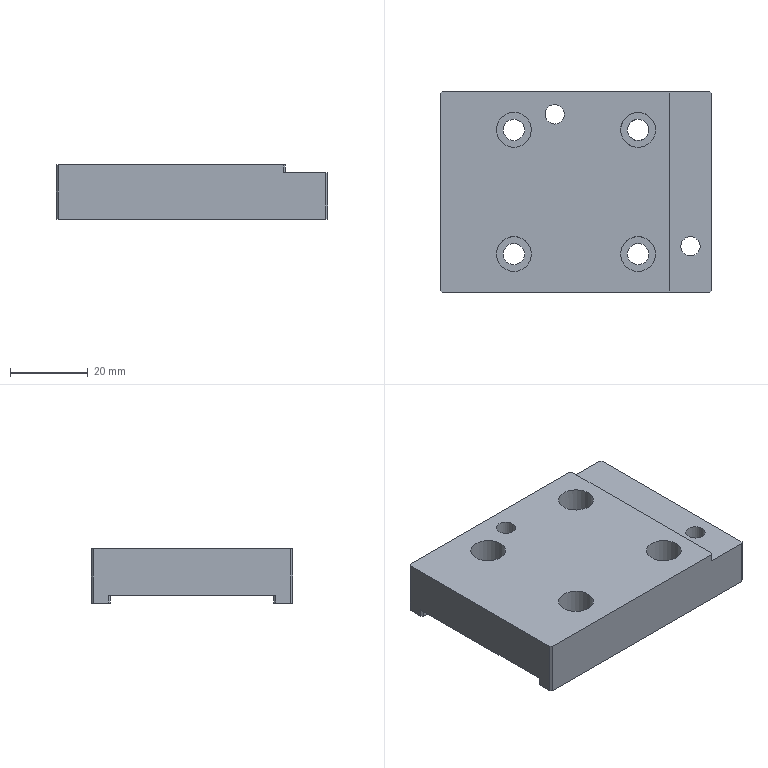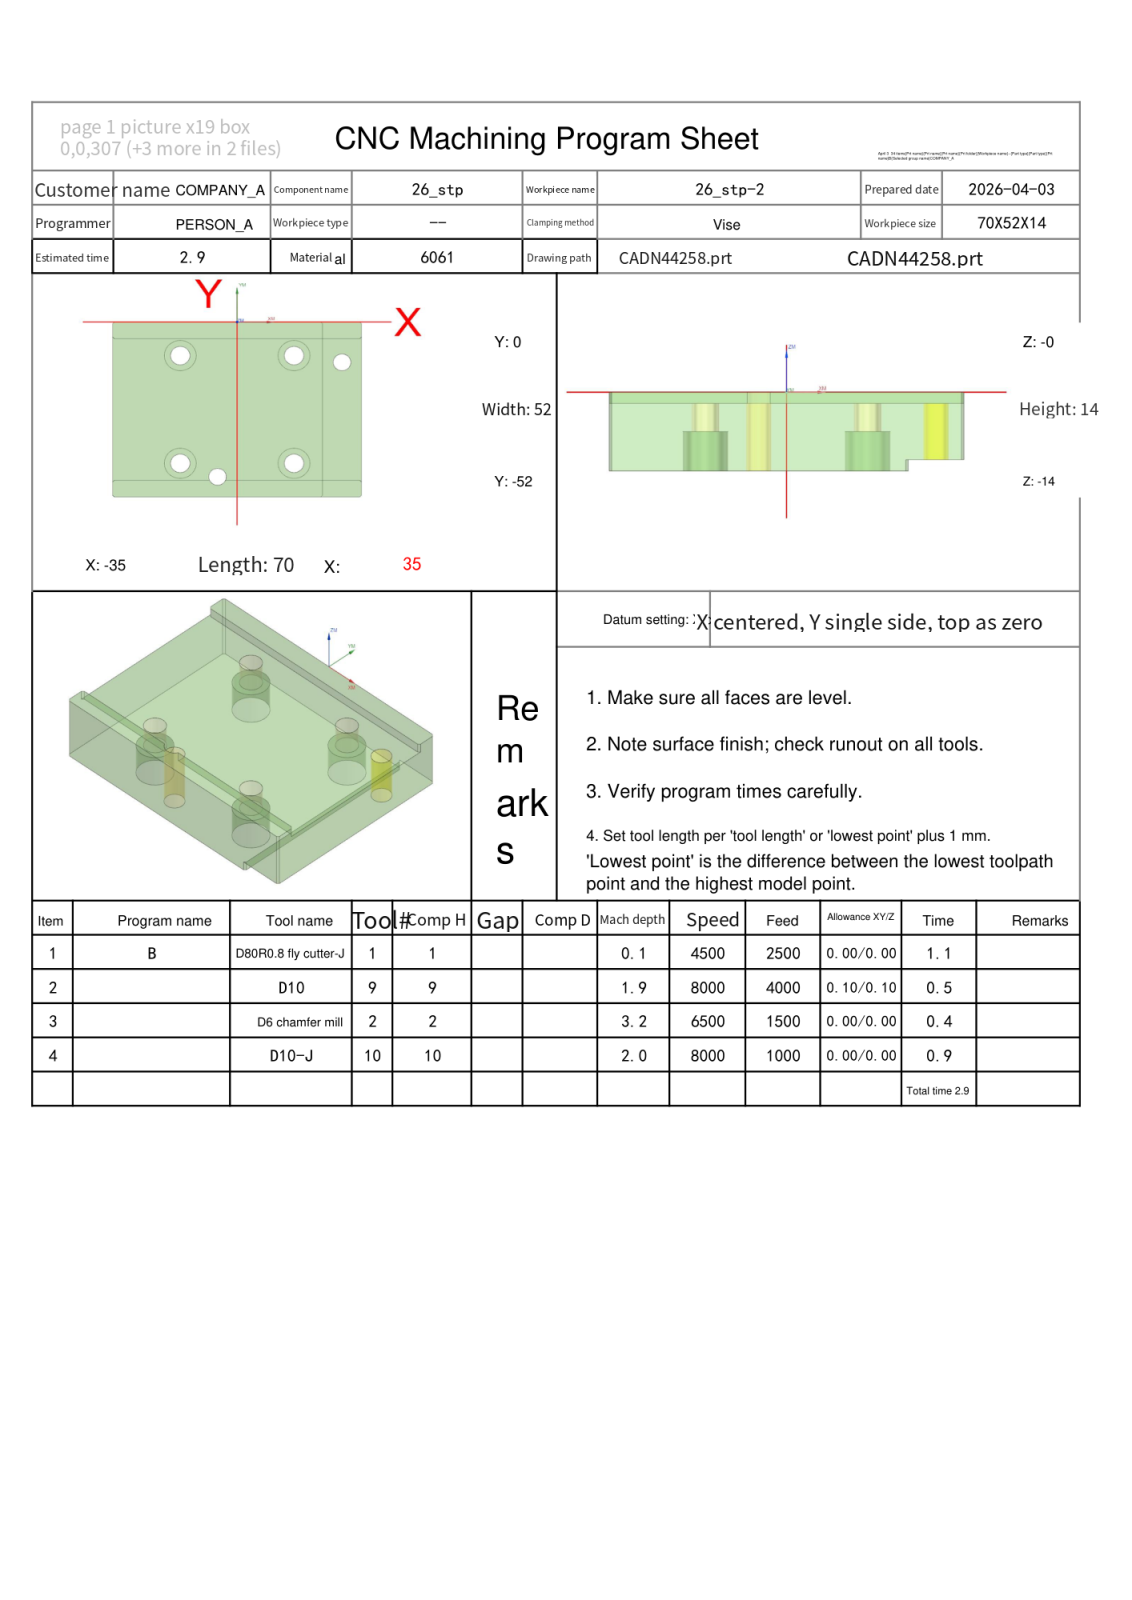NC program | NX | posted by the shop | part box 70 x 52 x 14 mm
Whole program:
%
O0001
(Machine time: 3.67 MIN)
(===Total Tool:4===)
(T1=D80R0.8 fly cutter-J D=80.  R=0.8  D-  H01 Z=-0.   )
(T9=D10     D=10.  R=0.   D-  H09 Z=-1.9  )
(T2=D6 chamfer mill   D=6.   R=0.   D-  H02 Z=-3.2  )
(T10=D10-J  D=10.  R=0.   D10 H10 Z=-2.   )
G80 G90 G17 G49 G40
G91 G28 Z0
M01
N1 T01 M06
(D80R0.8 fly cutter-J  D=80. R=0.8 H=01 ce=0.20 di=0.10)
G00 G90 G54 X87. Y-26. M03 S4500
G43 H01 Z20.
M08
Z7.009
G01 Z5.009 F2500.
X75.
X-75.
X-87.
Z7.009
G00 Z8.5
X87.
Z6.518
G01 Z4.518
X75.
X-75.
X-87.
Z6.518
G00 Z8.009
X87.
Z6.027
G01 Z4.027
X75.
X-75.
X-87.
Z6.027
G00 Z7.518
X87.
Z5.536
G01 Z3.536
X75.
X-75.
X-87.
Z5.536
G00 Z7.027
X87.
Z5.045
G01 Z3.045
X75.
X-75.
X-87.
Z5.045
G00 Z6.536
X87.
Z4.555
G01 Z2.555
X75.
X-75.
X-87.
Z4.555
G00 Z6.045
X87.
Z4.064
G01 Z2.064
X75.
X-75.
X-87.
Z4.064
G00 Z5.555
X87.
Z3.573
G01 Z1.573
X75.
X-75.
X-87.
Z3.573
G00 Z5.064
X87.
Z3.082
G01 Z1.082
X75.
X-75.
X-87.
Z3.082
G00 Z4.573
X87.
Z2.591
G01 Z.591
X75.
X-75.
X-87.
Z2.591
G00 Z4.082
X87.
Z2.1
G01 Z.1
X75.
X-75.
X-87.
Z2.1
G00 Z20.
G00 G90 X87. Y-26. M03 S4500
Z20.
Z2.
G01 Z0.0 F1000.
X75.
X-75.
X-87.
Z2.
G00 Z20.
G91 G28 Z0.0
M05
M09
G91 G28 Z0.0
M01
N2 T09 M06
(D10  D=10. R=0. H=09 ce=0.10 di=0.10)
G00 G90 G54 X43. Y-26. M03 S8000
G43 H09 Z15.502
M08
Z1.025
G01 Z-.475 F4000.
X39.9
Y-45.228
X36.612 Y-41.94
X-3.227
G03 X-5.5 Y-42.475 I0.0 J-5.1
X-7.773 Y-41.94 I-2.273 J-4.565
G01 X-36.612
X-39.9 Y-45.228
Y-6.772
X-36.612 Y-10.06
X36.612
X39.9 Y-6.772
Y-22.965
G02 X39.455 Y-23.797 I-1. J0.0
G01 X32.845 Y-28.203
G03 X32.4 Y-29.035 I.555 J-.832
G01 Y-33.442
G02 X31.402 Y-34.44 I-1. J.002
G01 X-3.227
G03 X-5.335 Y-34.618 I0.0 J-12.6
G01 X-5.5 Y-34.631
X-5.665 Y-34.618
G03 X-7.773 Y-34.44 I-2.108 J-12.422
G01 X-31.402
G02 X-32.4 Y-33.442 I.002 J1.
G01 Y-18.558
G02 X-31.402 Y-17.56 I1. J-.002
G01 X31.402
G02 X32.4 Y-18.558 I-.002 J-1.
G01 Y-22.783
G02 X31.721 Y-23.73 I-1. J0.0
G01 X25.413 Y-25.868
G03 X24.822 Y-26.407 I.321 J-.947
G02 X24.002 Y-26.94 I-.822 J.367
G01 X-3.227
G03 X-5.395 Y-27.057 I0.0 J-20.1
G01 X-5.5 Y-27.063
X-5.605 Y-27.057
G03 X-7.773 Y-26.94 I-2.168 J-19.983
G01 X-24.002
G02 X-24.9 Y-26.042 I.002 J.9
G01 Y-25.958
G02 X-24.002 Y-25.06 I.9 J-.002
G01 X24.002
G02 X24.901 Y-25.961 I-.002 J-.901
G01 X24.9 Y-26.
Y-26.042
G02 X24.785 Y-26.48 I-.9 J.002
G01 X27.402 Y-27.948
Z1.025
G00 X43. Y-26.
Z.55
G01 Z-.95
X39.9
Y-45.228
X36.612 Y-41.94
X-3.227
G03 X-5.5 Y-42.475 I0.0 J-5.1
X-7.773 Y-41.94 I-2.273 J-4.565
G01 X-36.612
X-39.9 Y-45.228
Y-6.772
X-36.612 Y-10.06
X36.612
X39.9 Y-6.772
Y-22.965
G02 X39.455 Y-23.797 I-1. J0.0
G01 X32.845 Y-28.203
G03 X32.4 Y-29.035 I.555 J-.832
G01 Y-33.442
G02 X31.402 Y-34.44 I-1. J.002
G01 X-3.227
G03 X-5.335 Y-34.618 I0.0 J-12.6
G01 X-5.5 Y-34.631
X-5.665 Y-34.618
G03 X-7.773 Y-34.44 I-2.108 J-12.422
G01 X-31.402
G02 X-32.4 Y-33.442 I.002 J1.
G01 Y-18.558
G02 X-31.402 Y-17.56 I1. J-.002
G01 X31.402
G02 X32.4 Y-18.558 I-.002 J-1.
G01 Y-22.783
G02 X31.721 Y-23.73 I-1. J0.0
G01 X25.413 Y-25.868
G03 X24.822 Y-26.407 I.321 J-.947
G02 X24.002 Y-26.94 I-.822 J.367
G01 X-3.227
G03 X-5.395 Y-27.057 I0.0 J-20.1
G01 X-5.5 Y-27.063
X-5.605 Y-27.057
G03 X-7.773 Y-26.94 I-2.168 J-19.983
G01 X-24.002
G02 X-24.9 Y-26.042 I.002 J.9
G01 Y-25.958
G02 X-24.002 Y-25.06 I.9 J-.002
G01 X24.002
G02 X24.901 Y-25.961 I-.002 J-.901
G01 X24.9 Y-26.
Y-26.042
G02 X24.785 Y-26.48 I-.9 J.002
G01 X27.402 Y-27.948
Z.55
G00 X43. Y-26.
Z.075
G01 Z-1.425
X39.9
Y-45.228
X36.612 Y-41.94
X-3.227
G03 X-5.5 Y-42.475 I0.0 J-5.1
X-7.773 Y-41.94 I-2.273 J-4.565
G01 X-36.612
X-39.9 Y-45.228
Y-6.772
X-36.612 Y-10.06
X36.612
X39.9 Y-6.772
Y-22.965
G02 X39.455 Y-23.797 I-1. J0.0
G01 X32.845 Y-28.203
G03 X32.4 Y-29.035 I.555 J-.832
G01 Y-33.442
G02 X31.402 Y-34.44 I-1. J.002
G01 X-3.227
G03 X-5.335 Y-34.618 I0.0 J-12.6
G01 X-5.5 Y-34.631
X-5.665 Y-34.618
G03 X-7.773 Y-34.44 I-2.108 J-12.422
G01 X-31.402
G02 X-32.4 Y-33.442 I.002 J1.
G01 Y-18.558
G02 X-31.402 Y-17.56 I1. J-.002
G01 X31.402
G02 X32.4 Y-18.558 I-.002 J-1.
G01 Y-22.783
G02 X31.721 Y-23.73 I-1. J0.0
G01 X25.413 Y-25.868
G03 X24.822 Y-26.407 I.321 J-.947
G02 X24.002 Y-26.94 I-.822 J.367
G01 X-3.227
G03 X-5.395 Y-27.057 I0.0 J-20.1
G01 X-5.5 Y-27.063
X-5.605 Y-27.057
G03 X-7.773 Y-26.94 I-2.168 J-19.983
G01 X-24.002
G02 X-24.9 Y-26.042 I.002 J.9
G01 Y-25.958
G02 X-24.002 Y-25.06 I.9 J-.002
G01 X24.002
G02 X24.901 Y-25.961 I-.002 J-.901
G01 X24.9 Y-26.
Y-26.042
G02 X24.785 Y-26.48 I-.9 J.002
G01 X27.402 Y-27.948
Z.075
G00 X43. Y-26.
Z-.4
G01 Z-1.9
X39.9
Y-45.228
X36.612 Y-41.94
X-3.227
G03 X-5.5 Y-42.475 I0.0 J-5.1
X-7.773 Y-41.94 I-2.273 J-4.565
G01 X-36.612
X-39.9 Y-45.228
Y-6.772
X-36.612 Y-10.06
X36.612
X39.9 Y-6.772
Y-22.965
G02 X39.455 Y-23.797 I-1. J0.0
G01 X32.845 Y-28.203
G03 X32.4 Y-29.035 I.555 J-.832
G01 Y-33.442
G02 X31.402 Y-34.44 I-1. J.002
G01 X-3.227
G03 X-5.335 Y-34.618 I0.0 J-12.6
G01 X-5.5 Y-34.631
X-5.665 Y-34.618
G03 X-7.773 Y-34.44 I-2.108 J-12.422
G01 X-31.402
G02 X-32.4 Y-33.442 I.002 J1.
G01 Y-18.558
G02 X-31.402 Y-17.56 I1. J-.002
G01 X31.402
G02 X32.4 Y-18.558 I-.002 J-1.
G01 Y-22.783
G02 X31.721 Y-23.73 I-1. J0.0
G01 X25.413 Y-25.868
G03 X24.822 Y-26.407 I.321 J-.947
G02 X24.002 Y-26.94 I-.822 J.367
G01 X-3.227
G03 X-5.395 Y-27.057 I0.0 J-20.1
G01 X-5.5 Y-27.063
X-5.605 Y-27.057
G03 X-7.773 Y-26.94 I-2.168 J-19.983
G01 X-24.002
G02 X-24.9 Y-26.042 I.002 J.9
G01 Y-25.958
G02 X-24.002 Y-25.06 I.9 J-.002
G01 X24.002
G02 X24.901 Y-25.961 I-.002 J-.901
G01 X24.9 Y-26.
Y-26.042
G02 X24.785 Y-26.48 I-.9 J.002
G01 X27.402 Y-27.948
Z-.4
G00 Z15.502
G91 G28 Z0.0
M05
M09
G91 G28 Z0.0
M01
N3 T02 M06
(D6 chamfer mill  D=6. R=0. H=02 ce=0.00 di=0.00)
G00 G90 G54 X.386 Y-53.227 M03 S6500
G43 H02 Z20.
M08
Z.172
G01 Z-1.199 F1500.
G03 X.1 Y-53.027 I-1.286 J-1.532
G01 X.054 Y-52.997
X0.0 Y-53.
X-34.5
X-34.759 Y-52.966
X-35. Y-52.866
X-35.207 Y-52.707
X-35.707 Y-52.207
X-35.866 Y-52.
X-35.966 Y-51.759
X-36. Y-51.5
Y-47.54
X-35.966 Y-47.281
X-35.866 Y-47.04
X-35.707 Y-46.833
X-35.207 Y-46.333
X-35. Y-46.174
X-34.759 Y-46.074
X-34.5 Y-46.04
X-7.773
X-7.547 Y-46.066
X-7.332 Y-46.142
X-7.141 Y-46.266
X-6.982 Y-46.429
X-6.687 Y-46.917
G03 X-5.5 Y-47.5 I1.187 J.917
X-4.313 Y-46.917 I0.0 J1.5
G01 X-4.018 Y-46.429
X-3.859 Y-46.266
X-3.668 Y-46.142
X-3.453 Y-46.066
X-3.227 Y-46.04
X34.5
X34.759 Y-46.074
X35. Y-46.174
X35.207 Y-46.333
X35.707 Y-46.833
X35.866 Y-47.04
X35.966 Y-47.281
X36. Y-47.54
Y-51.5
X35.966 Y-51.759
X35.866 Y-52.
X35.707 Y-52.207
X35.207 Y-52.707
X35. Y-52.866
X34.759 Y-52.966
X34.5 Y-53.
X0.0
X-.054 Y-52.997
X-.1 Y-53.027
G03 X-.386 Y-53.227 I1. J-1.732
G01 Z.172
G00 Z10.
X.386 Y-6.187
Z.172
G01 Z-1.199
G03 X.1 Y-5.987 I-1.286 J-1.532
G01 X.054 Y-5.957
X0.0 Y-5.96
X-34.5
X-34.759 Y-5.926
X-35. Y-5.826
X-35.207 Y-5.667
X-35.707 Y-5.167
X-35.866 Y-4.96
X-35.966 Y-4.719
X-36. Y-4.46
Y-.5
X-35.966 Y-.241
X-35.866 Y0.0
X-35.707 Y.207
X-35.207 Y.707
X-35. Y.866
X-34.759 Y.966
X-34.5 Y1.
X34.5
X34.759 Y.966
X35. Y.866
X35.207 Y.707
X35.707 Y.207
X35.866 Y0.0
X35.966 Y-.241
X36. Y-.5
Y-4.46
X35.966 Y-4.719
X35.866 Y-4.96
X35.707 Y-5.167
X35.207 Y-5.667
X35. Y-5.826
X34.759 Y-5.926
X34.5 Y-5.96
X0.0
X-.054 Y-5.957
X-.1 Y-5.987
G03 X-.386 Y-6.187 I1. J-1.732
G01 Z.172
G00 Z10.
X-5.222 Y-44.577
Z-1.645
G01 Z-3.199
X-5.274 Y-44.531
X-5.293 Y-44.523
X-5.5 Y-44.5
X-5.707 Y-44.523
X-5.726 Y-44.531
X-5.778 Y-44.577
Z-1.645
G00 Z10.
X36.113 Y-7.675
Z-1.715
G01 Z-3.199
X36.052 Y-7.738
X36.013 Y-7.818
X35.994 Y-7.839
X36. Y-7.868
Y-44.132
X35.994 Y-44.161
X36.013 Y-44.182
X36.052 Y-44.262
X36.113 Y-44.325
Z-1.715
G00 Z10.
X-36.113
Z-1.715
G01 Z-3.199
X-36.052 Y-44.262
X-36.013 Y-44.182
X-35.994 Y-44.161
X-36. Y-44.132
Y-7.868
X-35.994 Y-7.839
X-36.013 Y-7.818
X-36.052 Y-7.738
X-36.113 Y-7.675
Z-1.715
G00 Z10.
X30.815 Y-12.407
Z-1.716
G01 Z-3.199
G03 X30.984 Y-12.102 I-1.658 J1.118
G01 X31.009 Y-12.054
X31. Y-12.
G03 X29.5 Y-10.5 I-1.5 J0.0
X28. Y-12. I0.0 J-1.5
X29.5 Y-13.5 I1.5 J0.0
X31. Y-12. I0.0 J1.5
G01 X31.009 Y-11.946
X30.984 Y-11.898
G03 X30.815 Y-11.593 I-1.827 J-.813
G01 Z-1.716
G00 Z10.
X14.435 Y-9.593
Z-1.73
G01 Z-3.199
G03 X14.266 Y-9.898 I1.658 J-1.118
G01 X14.241 Y-9.946
X14.25 Y-10.
G03 X16. Y-11.75 I1.75 J0.0
X17.75 Y-10. I0.0 J1.75
X16. Y-8.25 I-1.75 J0.0
X14.25 Y-10. I0.0 J-1.75
G01 X14.241 Y-10.054
X14.266 Y-10.102
G03 X14.435 Y-10.407 I1.827 J.813
G01 Z-1.73
G00 Z10.
Y-41.593
Z-1.73
G01 Z-3.199
G03 X14.266 Y-41.898 I1.658 J-1.118
G01 X14.241 Y-41.946
X14.25 Y-42.
G03 X16. Y-43.75 I1.75 J0.0
X17.75 Y-42. I0.0 J1.75
X16. Y-40.25 I-1.75 J0.0
X14.25 Y-42. I0.0 J-1.75
G01 X14.241 Y-42.054
X14.266 Y-42.102
G03 X14.435 Y-42.407 I1.827 J.813
G01 Z-1.73
G00 Z10.
X-17.565 Y-41.593
Z-1.73
G01 Z-3.199
G03 X-17.734 Y-41.898 I1.658 J-1.118
G01 X-17.759 Y-41.946
X-17.75 Y-42.
G03 X-16. Y-43.75 I1.75 J0.0
X-14.25 Y-42. I0.0 J1.75
X-16. Y-40.25 I-1.75 J0.0
X-17.75 Y-42. I0.0 J-1.75
G01 X-17.759 Y-42.054
X-17.734 Y-42.102
G03 X-17.565 Y-42.407 I1.827 J.813
G01 Z-1.73
G00 Z10.
Y-9.593
Z-1.73
G01 Z-3.199
G03 X-17.734 Y-9.898 I1.658 J-1.118
G01 X-17.759 Y-9.946
X-17.75 Y-10.
G03 X-16. Y-11.75 I1.75 J0.0
X-14.25 Y-10. I0.0 J1.75
X-16. Y-8.25 I-1.75 J0.0
X-17.75 Y-10. I0.0 J-1.75
G01 X-17.759 Y-10.054
X-17.734 Y-10.102
G03 X-17.565 Y-10.407 I1.827 J.813
G01 Z-1.73
G00 Z20.
G91 G28 Z0.0
M05
M09
G91 G28 Z0.0
M01
N4 T10 M06
(D10-J  D=10. R=0. H=10 ce=0.40 di=0.00)
G00 G90 G54 X42. Y-43.639 M03 S8000
G43 H10 Z15.502
M08
Z-.5
G01 Z-2. F1000.
G03 X40. Y-41.639 I-2. J0.0
G01 X-39.1
G02 X-40. Y-40.739 I0.0 J.9
G01 Y-38.171
G02 X-39. Y-37.171 I1. J0.0
G01 X39.1
G03 X40. Y-36.271 I0.0 J.9
G01 Y-33.702
G03 X39. Y-32.702 I-1. J0.0
G01 X-39.
G02 X-40. Y-31.702 I0.0 J1.
G01 Y-29.134
G02 X-39.1 Y-28.234 I.9 J0.0
G01 X39.1
G03 X40. Y-27.334 I0.0 J.9
G01 Y-24.765
G03 X39. Y-23.765 I-1. J0.0
G01 X-39.1
G02 X-40. Y-22.865 I0.0 J.9
G01 Y-20.297
G02 X-39. Y-19.297 I1. J0.0
G01 X39.1
G03 X40. Y-18.397 I0.0 J.9
G01 Y-15.828
G03 X39. Y-14.828 I-1. J0.0
G01 X-39.1
G02 X-40. Y-13.928 I0.0 J.9
G01 Y-11.36
G02 X-39. Y-10.36 I1. J0.0
G01 X40.
G02 X42. Y-12.36 I0.0 J-2.
G01 Z-.5
G00 Z15.502
G00 G90 X42.191 Y-6.092 M03 S8000
Z15.502
Z-1.
G01 Z-2. F1000.
G41 D10
X42. Y-6.033
G03 X41.414 Y-5.945 I-.586 J-1.912
X40. Y-6.531 I0.0 J-2.
G01 X36.571 Y-9.96
X-36.571
X-40. Y-6.531
G03 X-41.414 Y-5.945 I-1.414 J-1.414
X-42. Y-6.033 I0.0 J-2.
G01 G40 X-42.191 Y-6.092
Z-1.
G00 Y-45.908
G01 Z-2.
G41 D10
X-42. Y-45.967
G03 X-41.414 Y-46.055 I.586 J1.912
X-40. Y-45.469 I0.0 J2.
G01 X-36.571 Y-42.04
X36.571
X40. Y-45.469
G03 X41.414 Y-46.055 I1.414 J1.414
X42. Y-45.967 I0.0 J2.
G01 G40 X42.191 Y-45.908
Z-1.
G00 Z15.502
M05
M09
G91 G28 Z0.0
G91 G28 Y0.0
M30
%